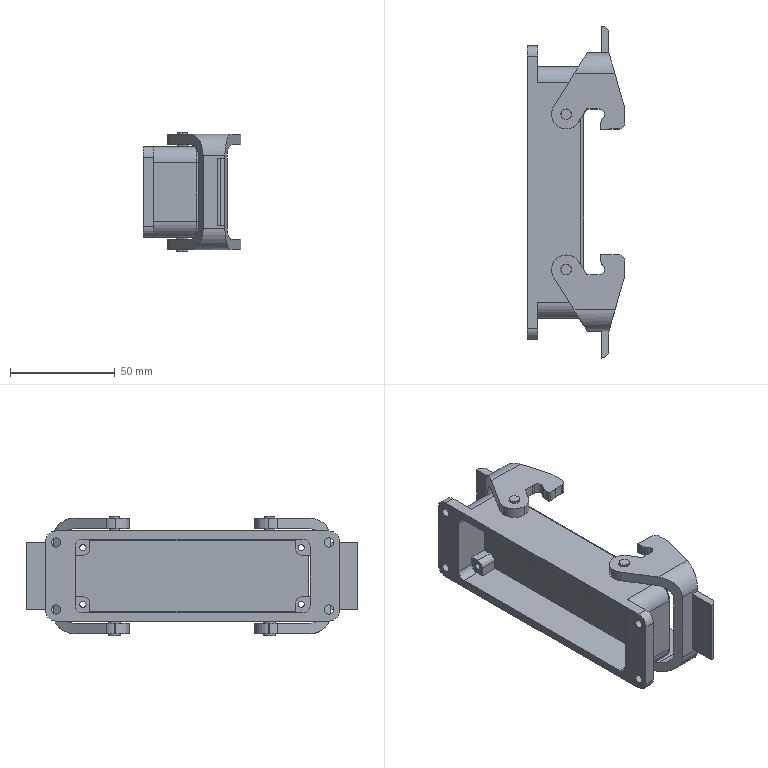Part | STEP file | 4-20.sldasm-Part-9 | 1 solid | 271 faces | box 46.6 x 158.128 x 57 mm | volume 96825 mm3 | plane 137 | cylinder 126 | torus 8 | commonest cylinder face diameters 2 x20 7 x12 3 x8 3.3 x8 4.4 x8 5.5 x8